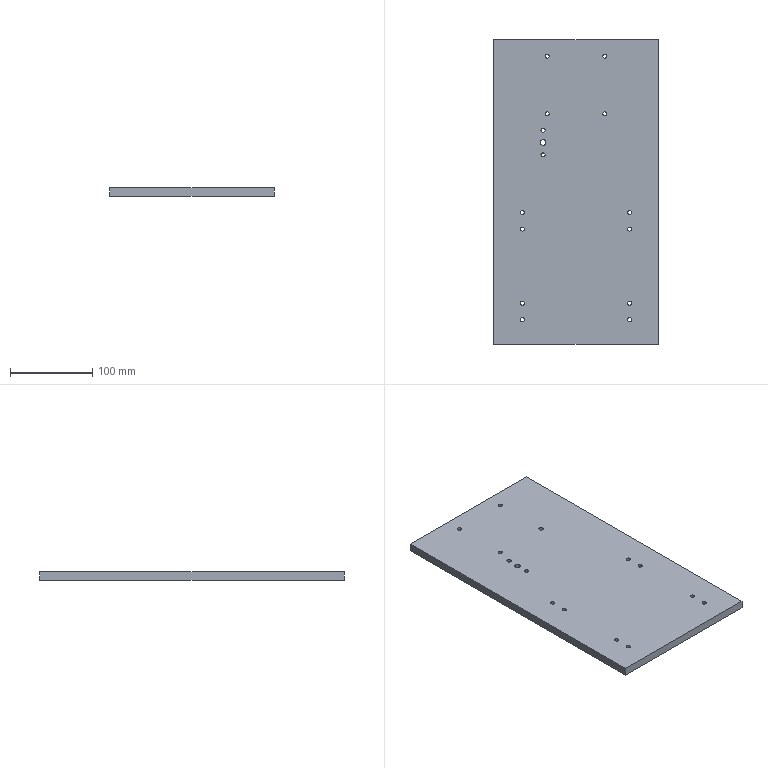Part | STEP file | 0217_205_Base_Plate | 1 solid | 36 faces | box 200 x 370 x 10 mm | volume 736866 mm3 | cylinder 30 | plane 6 | commonest cylinder face diameters 5 x28 7 x2